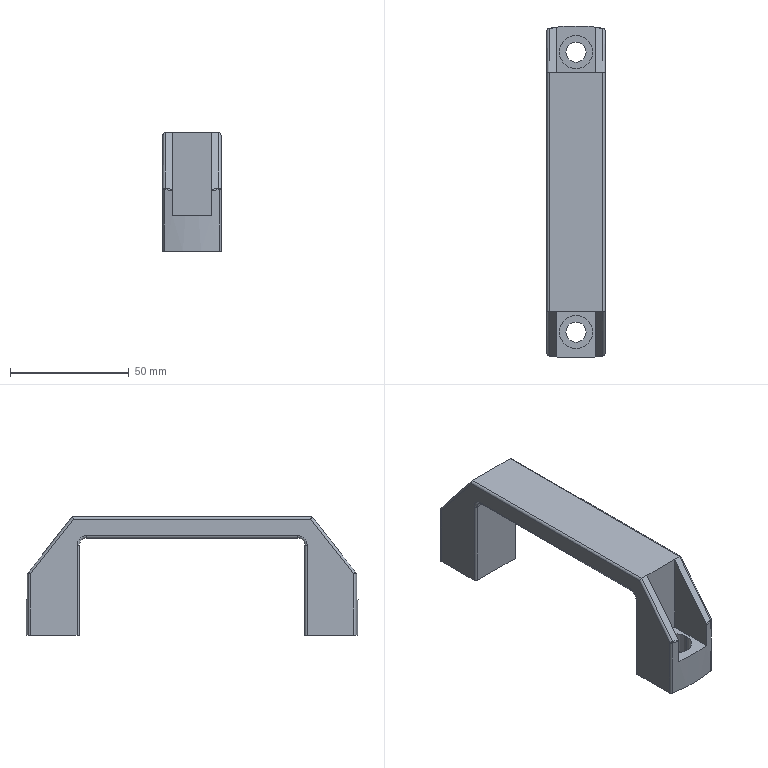Part | NX | features BREP 1 | 1 solid | 63 faces | box 24.5 x 140 x 50 mm | volume 45772 mm3 | cylinder 29 | plane 22 | torus 4 | spline 4 | sphere 4 | commonest cylinder face diameters 2 x16 8.5 x4 14 x4 140 x3 6 x2